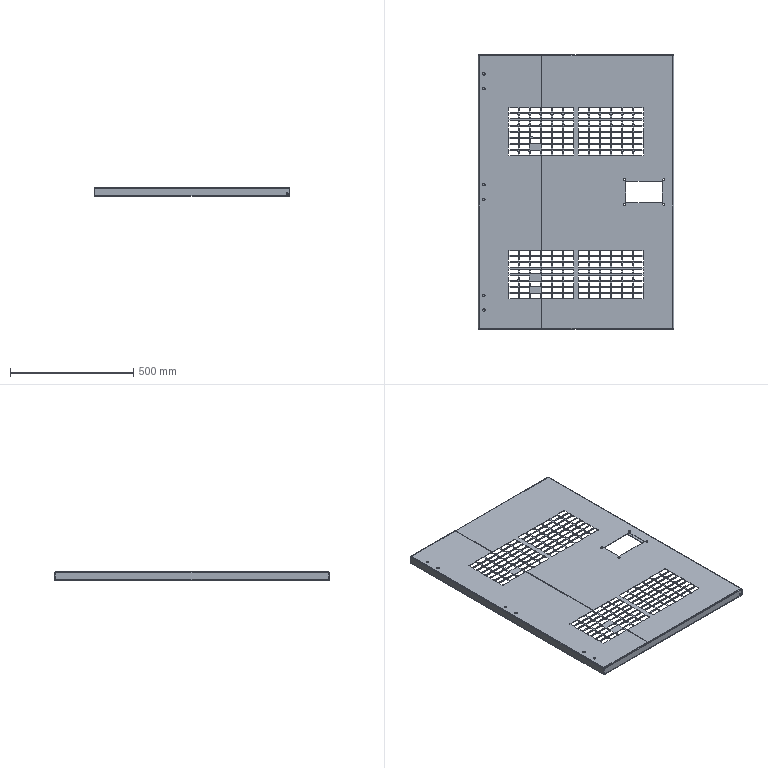Part | STEP file | SYL_0392D6J1SYL0380DJ10-1155504 | 1 solid | 1711 faces | box 794 x 1114 x 35 mm | volume 1839649 mm3 | plane 902 | spline 793 | cylinder 16 | commonest cylinder face diameters 4 x8 8 x8